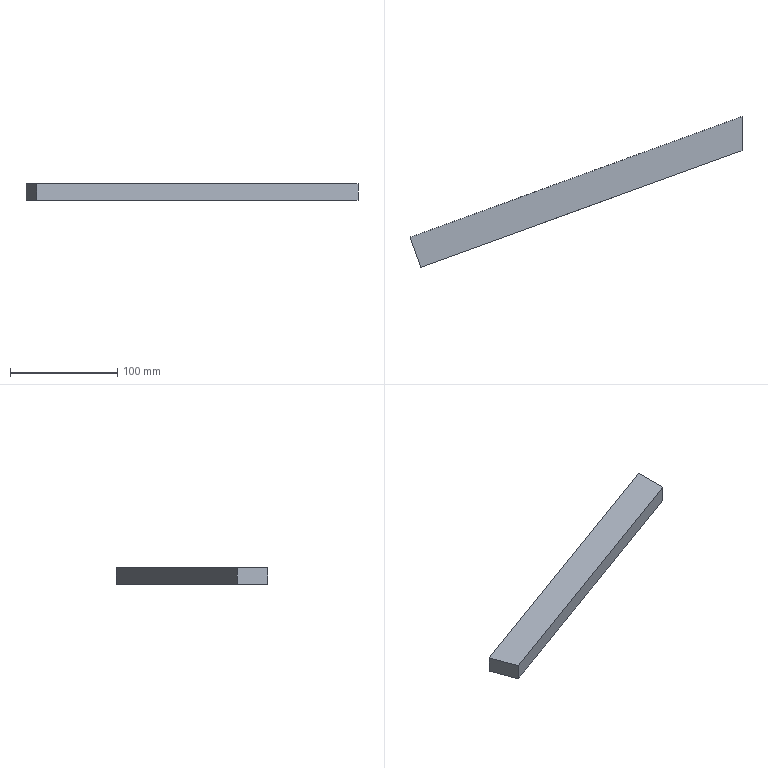Part | NX | features solid 2 | 1 solid | 6 faces | box 310.099 x 141.057 x 15 mm | volume 146043 mm3 | plane 6
STEP:
#1=CARTESIAN_POINT('',(680.,-281.925,-45.));
#2=VERTEX_POINT('',#1);
#3=CARTESIAN_POINT('',(680.,-281.925,-30.));
#4=VERTEX_POINT('',#3);
#5=CARTESIAN_POINT('',(680.,-281.925,-45.));
#6=DIRECTION('',(0.,0.,-1.));
#7=VECTOR('',#6,1000.);
#8=LINE('',#5,#7);
#9=EDGE_CURVE('',#2,#4,#8,.F.);
#10=ORIENTED_EDGE('',*,*,#9,.T.);
#11=CARTESIAN_POINT('',(380.162,-391.057,-30.));
#12=VERTEX_POINT('',#11);
#13=CARTESIAN_POINT('',(690.261,-278.191,-30.));
#14=DIRECTION('',(-0.9397,-0.342,0.));
#15=VECTOR('',#14,1000.);
#16=LINE('',#13,#15);
#17=EDGE_CURVE('',#4,#12,#16,.T.);
#18=ORIENTED_EDGE('',*,*,#17,.T.);
#19=CARTESIAN_POINT('',(380.162,-391.057,-45.));
#20=VERTEX_POINT('',#19);
#21=CARTESIAN_POINT('',(380.162,-391.057,-45.));
#22=DIRECTION('',(0.,0.,1.));
#23=VECTOR('',#22,1000.);
#24=LINE('',#21,#23);
#25=EDGE_CURVE('',#20,#12,#24,.T.);
#26=ORIENTED_EDGE('',*,*,#25,.F.);
#27=CARTESIAN_POINT('',(690.261,-278.191,-45.));
#28=DIRECTION('',(-0.9397,-0.342,0.));
#29=VECTOR('',#28,1000.);
#30=LINE('',#27,#29);
#31=EDGE_CURVE('',#2,#20,#30,.T.);
#32=ORIENTED_EDGE('',*,*,#31,.F.);
#33=EDGE_LOOP('',(#10,#18,#26,#32));
#34=FACE_BOUND('',#33,.T.);
#35=CARTESIAN_POINT('',(690.261,-278.191,-45.));
#36=DIRECTION('',(0.342,-0.9397,0.));
#37=DIRECTION('',(-0.9397,-0.342,0.));
#38=AXIS2_PLACEMENT_3D('',#35,#36,#37);
#39=PLANE('',#38);
#40=ADVANCED_FACE('',(#34),#39,.T.);
#41=ORIENTED_EDGE('',*,*,#25,.T.);
#42=CARTESIAN_POINT('',(369.901,-362.867,-30.));
#43=VERTEX_POINT('',#42);
#44=CARTESIAN_POINT('',(380.162,-391.057,-30.));
#45=DIRECTION('',(0.342,-0.9397,0.));
#46=VECTOR('',#45,1000.);
#47=LINE('',#44,#46);
#48=EDGE_CURVE('',#12,#43,#47,.F.);
#49=ORIENTED_EDGE('',*,*,#48,.T.);
#50=CARTESIAN_POINT('',(369.901,-362.867,-45.));
#51=VERTEX_POINT('',#50);
#52=CARTESIAN_POINT('',(369.901,-362.867,-45.));
#53=DIRECTION('',(0.,0.,-1.));
#54=VECTOR('',#53,1000.);
#55=LINE('',#52,#54);
#56=EDGE_CURVE('',#51,#43,#55,.F.);
#57=ORIENTED_EDGE('',*,*,#56,.F.);
#58=CARTESIAN_POINT('',(380.162,-391.057,-45.));
#59=DIRECTION('',(0.342,-0.9397,0.));
#60=VECTOR('',#59,1000.);
#61=LINE('',#58,#60);
#62=EDGE_CURVE('',#20,#51,#61,.F.);
#63=ORIENTED_EDGE('',*,*,#62,.F.);
#64=EDGE_LOOP('',(#41,#49,#57,#63));
#65=FACE_BOUND('',#64,.T.);
#66=CARTESIAN_POINT('',(380.162,-391.057,-45.));
#67=DIRECTION('',(-0.9397,-0.342,0.));
#68=DIRECTION('',(-0.342,0.9397,0.));
#69=AXIS2_PLACEMENT_3D('',#66,#67,#68);
#70=PLANE('',#69);
#71=ADVANCED_FACE('',(#65),#70,.T.);
#72=ORIENTED_EDGE('',*,*,#56,.T.);
#73=CARTESIAN_POINT('',(680.,-250.,-30.));
#74=VERTEX_POINT('',#73);
#75=CARTESIAN_POINT('',(680.,-250.,-30.));
#76=DIRECTION('',(-0.9397,-0.342,0.));
#77=VECTOR('',#76,1000.);
#78=LINE('',#75,#77);
#79=EDGE_CURVE('',#74,#43,#78,.T.);
#80=ORIENTED_EDGE('',*,*,#79,.F.);
#81=CARTESIAN_POINT('',(680.,-250.,-45.));
#82=VERTEX_POINT('',#81);
#83=CARTESIAN_POINT('',(680.,-250.,-70.));
#84=DIRECTION('',(0.,0.,1.));
#85=VECTOR('',#84,1000.);
#86=LINE('',#83,#85);
#87=EDGE_CURVE('',#82,#74,#86,.T.);
#88=ORIENTED_EDGE('',*,*,#87,.F.);
#89=CARTESIAN_POINT('',(680.,-250.,-45.));
#90=DIRECTION('',(-0.9397,-0.342,0.));
#91=VECTOR('',#90,1000.);
#92=LINE('',#89,#91);
#93=EDGE_CURVE('',#82,#51,#92,.T.);
#94=ORIENTED_EDGE('',*,*,#93,.T.);
#95=EDGE_LOOP('',(#72,#80,#88,#94));
#96=FACE_BOUND('',#95,.T.);
#97=CARTESIAN_POINT('',(680.,-250.,-45.));
#98=DIRECTION('',(0.342,-0.9397,0.));
#99=DIRECTION('',(-0.9397,-0.342,0.));
#100=AXIS2_PLACEMENT_3D('',#97,#98,#99);
#101=PLANE('',#100);
#102=ADVANCED_FACE('',(#96),#101,.F.);
#103=CARTESIAN_POINT('',(680.,-278.191,-45.));
#104=DIRECTION('',(0.,1.,0.));
#105=VECTOR('',#104,1000.);
#106=LINE('',#103,#105);
#107=EDGE_CURVE('',#2,#82,#106,.T.);
#108=ORIENTED_EDGE('',*,*,#107,.T.);
#109=ORIENTED_EDGE('',*,*,#87,.T.);
#110=CARTESIAN_POINT('',(680.,-278.191,-30.));
#111=DIRECTION('',(0.,1.,0.));
#112=VECTOR('',#111,1000.);
#113=LINE('',#110,#112);
#114=EDGE_CURVE('',#4,#74,#113,.T.);
#115=ORIENTED_EDGE('',*,*,#114,.F.);
#116=ORIENTED_EDGE('',*,*,#9,.F.);
#117=EDGE_LOOP('',(#108,#109,#115,#116));
#118=FACE_BOUND('',#117,.T.);
#119=CARTESIAN_POINT('',(680.,-25.,-70.));
#120=DIRECTION('',(-1.,0.,0.));
#121=DIRECTION('',(0.,-1.,0.));
#122=AXIS2_PLACEMENT_3D('',#119,#120,#121);
#123=PLANE('',#122);
#124=ADVANCED_FACE('',(#118),#123,.F.);
#125=ORIENTED_EDGE('',*,*,#79,.T.);
#126=ORIENTED_EDGE('',*,*,#48,.F.);
#127=ORIENTED_EDGE('',*,*,#17,.F.);
#128=ORIENTED_EDGE('',*,*,#114,.T.);
#129=EDGE_LOOP('',(#125,#126,#127,#128));
#130=FACE_BOUND('',#129,.T.);
#131=CARTESIAN_POINT('',(690.261,-278.191,-30.));
#132=DIRECTION('',(0.,0.,-1.));
#133=DIRECTION('',(-0.9397,-0.342,0.));
#134=AXIS2_PLACEMENT_3D('',#131,#132,#133);
#135=PLANE('',#134);
#136=ADVANCED_FACE('',(#130),#135,.F.);
#137=ORIENTED_EDGE('',*,*,#93,.F.);
#138=ORIENTED_EDGE('',*,*,#107,.F.);
#139=ORIENTED_EDGE('',*,*,#31,.T.);
#140=ORIENTED_EDGE('',*,*,#62,.T.);
#141=EDGE_LOOP('',(#137,#138,#139,#140));
#142=FACE_BOUND('',#141,.T.);
#143=CARTESIAN_POINT('',(690.261,-278.191,-45.));
#144=DIRECTION('',(0.,0.,-1.));
#145=DIRECTION('',(-0.9397,-0.342,0.));
#146=AXIS2_PLACEMENT_3D('',#143,#144,#145);
#147=PLANE('',#146);
#148=ADVANCED_FACE('',(#142),#147,.T.);
#149=CLOSED_SHELL('',(#40,#71,#102,#124,#136,#148));
#150=MANIFOLD_SOLID_BREP('',#149);
#151=(LENGTH_UNIT()NAMED_UNIT(*)SI_UNIT(.MILLI.,.METRE.));
#152=UNCERTAINTY_MEASURE_WITH_UNIT(LENGTH_MEASURE(0.00001),#151,'','');
#153=(NAMED_UNIT(*)PLANE_ANGLE_UNIT()SI_UNIT($,.RADIAN.));
#154=(NAMED_UNIT(*)SI_UNIT($,.STERADIAN.)SOLID_ANGLE_UNIT());
#155=(GEOMETRIC_REPRESENTATION_CONTEXT(3)GLOBAL_UNCERTAINTY_ASSIGNED_CONTEXT((#152))GLOBAL_UNIT_ASSIGNED_CONTEXT((#151,#153,#154))REPRESENTATION_CONTEXT('',''));
#156=ADVANCED_BREP_SHAPE_REPRESENTATION('',(#150),#155);